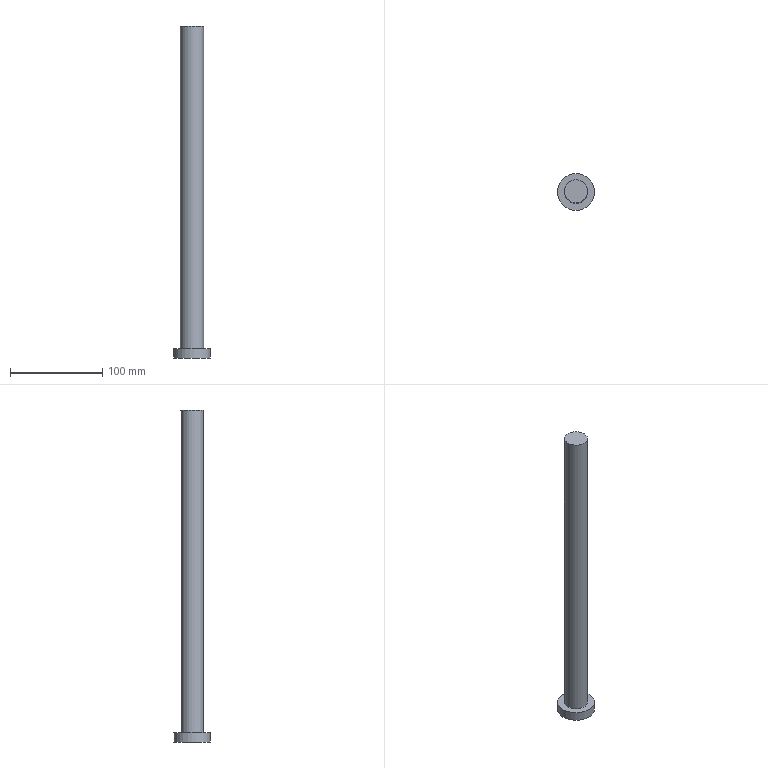Part | NX | features 护邦销 2 | 1 solid | 5 faces | box 40 x 40 x 360 mm | volume 184372 mm3 | plane 3 | cylinder 2 | commonest cylinder face diameters 25 x1 40 x1
STEP:
#1=CARTESIAN_POINT('',(12.5,0.,350.));
#2=VERTEX_POINT('',#1);
#3=CARTESIAN_POINT('',(0.,0.,350.));
#4=DIRECTION('',(0.,0.,1.));
#5=DIRECTION('',(1.,0.,0.));
#6=AXIS2_PLACEMENT_3D('',#3,#4,#5);
#7=CIRCLE('',#6,12.5);
#8=EDGE_CURVE('',#2,#2,#7,.T.);
#9=ORIENTED_EDGE('',*,*,#8,.F.);
#10=EDGE_LOOP('',(#9));
#11=FACE_BOUND('',#10,.T.);
#12=CARTESIAN_POINT('',(-12.5,0.,0.));
#13=VERTEX_POINT('',#12);
#14=CARTESIAN_POINT('',(0.,0.,0.));
#15=DIRECTION('',(0.,0.,-1.));
#16=DIRECTION('',(-1.,0.,0.));
#17=AXIS2_PLACEMENT_3D('',#14,#15,#16);
#18=CIRCLE('',#17,12.5);
#19=EDGE_CURVE('',#13,#13,#18,.T.);
#20=ORIENTED_EDGE('',*,*,#19,.F.);
#21=EDGE_LOOP('',(#20));
#22=FACE_BOUND('',#21,.T.);
#23=CARTESIAN_POINT('',(0.,0.,350.));
#24=DIRECTION('',(0.,0.,-1.));
#25=DIRECTION('',(-1.,0.,0.));
#26=AXIS2_PLACEMENT_3D('',#23,#24,#25);
#27=CYLINDRICAL_SURFACE('',#26,12.5);
#28=ADVANCED_FACE('',(#11,#22),#27,.T.);
#29=ORIENTED_EDGE('',*,*,#8,.T.);
#30=EDGE_LOOP('',(#29));
#31=FACE_BOUND('',#30,.T.);
#32=CARTESIAN_POINT('',(0.,0.,350.));
#33=DIRECTION('',(0.,0.,1.));
#34=DIRECTION('',(1.,0.,0.));
#35=AXIS2_PLACEMENT_3D('',#32,#33,#34);
#36=PLANE('',#35);
#37=ADVANCED_FACE('',(#31),#36,.T.);
#38=CARTESIAN_POINT('',(-20.,0.,0.));
#39=VERTEX_POINT('',#38);
#40=CARTESIAN_POINT('',(0.,0.,0.));
#41=DIRECTION('',(0.,0.,-1.));
#42=DIRECTION('',(-1.,0.,0.));
#43=AXIS2_PLACEMENT_3D('',#40,#41,#42);
#44=CIRCLE('',#43,20.);
#45=EDGE_CURVE('',#39,#39,#44,.T.);
#46=ORIENTED_EDGE('',*,*,#45,.F.);
#47=EDGE_LOOP('',(#46));
#48=FACE_BOUND('',#47,.T.);
#49=ORIENTED_EDGE('',*,*,#19,.T.);
#50=EDGE_LOOP('',(#49));
#51=FACE_BOUND('',#50,.T.);
#52=CARTESIAN_POINT('',(0.,0.,0.));
#53=DIRECTION('',(0.,0.,-1.));
#54=DIRECTION('',(-1.,0.,0.));
#55=AXIS2_PLACEMENT_3D('',#52,#53,#54);
#56=PLANE('',#55);
#57=ADVANCED_FACE('',(#48,#51),#56,.F.);
#58=CARTESIAN_POINT('',(-20.,0.,-10.));
#59=VERTEX_POINT('',#58);
#60=CARTESIAN_POINT('',(0.,0.,-10.));
#61=DIRECTION('',(0.,0.,-1.));
#62=DIRECTION('',(-1.,0.,0.));
#63=AXIS2_PLACEMENT_3D('',#60,#61,#62);
#64=CIRCLE('',#63,20.);
#65=EDGE_CURVE('',#59,#59,#64,.T.);
#66=ORIENTED_EDGE('',*,*,#65,.F.);
#67=EDGE_LOOP('',(#66));
#68=FACE_BOUND('',#67,.T.);
#69=ORIENTED_EDGE('',*,*,#45,.T.);
#70=EDGE_LOOP('',(#69));
#71=FACE_BOUND('',#70,.T.);
#72=CARTESIAN_POINT('',(0.,0.,-10.));
#73=DIRECTION('',(0.,0.,1.));
#74=DIRECTION('',(1.,0.,0.));
#75=AXIS2_PLACEMENT_3D('',#72,#73,#74);
#76=CYLINDRICAL_SURFACE('',#75,20.);
#77=ADVANCED_FACE('',(#68,#71),#76,.T.);
#78=ORIENTED_EDGE('',*,*,#65,.T.);
#79=EDGE_LOOP('',(#78));
#80=FACE_BOUND('',#79,.T.);
#81=CARTESIAN_POINT('',(0.,0.,-10.));
#82=DIRECTION('',(0.,0.,-1.));
#83=DIRECTION('',(-1.,0.,0.));
#84=AXIS2_PLACEMENT_3D('',#81,#82,#83);
#85=PLANE('',#84);
#86=ADVANCED_FACE('',(#80),#85,.T.);
#87=CLOSED_SHELL('',(#28,#37,#57,#77,#86));
#88=MANIFOLD_SOLID_BREP('',#87);
#89=(LENGTH_UNIT()NAMED_UNIT(*)SI_UNIT(.MILLI.,.METRE.));
#90=UNCERTAINTY_MEASURE_WITH_UNIT(LENGTH_MEASURE(0.00001),#89,'','');
#91=(NAMED_UNIT(*)PLANE_ANGLE_UNIT()SI_UNIT($,.RADIAN.));
#92=(NAMED_UNIT(*)SI_UNIT($,.STERADIAN.)SOLID_ANGLE_UNIT());
#93=(GEOMETRIC_REPRESENTATION_CONTEXT(3)GLOBAL_UNCERTAINTY_ASSIGNED_CONTEXT((#90))GLOBAL_UNIT_ASSIGNED_CONTEXT((#89,#91,#92))REPRESENTATION_CONTEXT('',''));
#94=ADVANCED_BREP_SHAPE_REPRESENTATION('',(#88),#93);